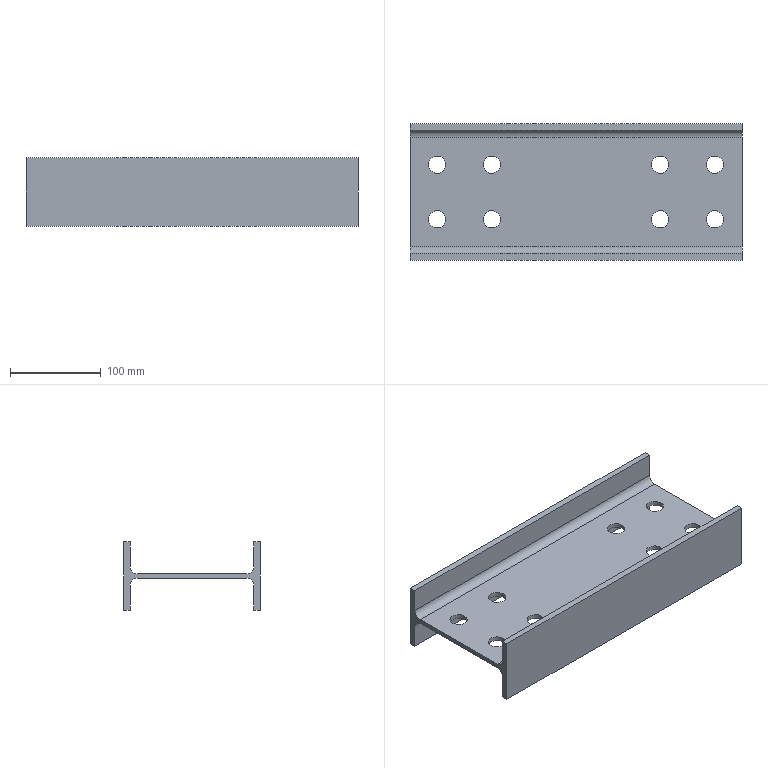Part | STEP file | Powder bin secondary beam 2_Default<As Machined> | 1 solid | 34 faces | box 365 x 150 x 75 mm | volume 640161 mm3 | cylinder 20 | plane 14 | commonest cylinder face diameters 19 x16 16 x4